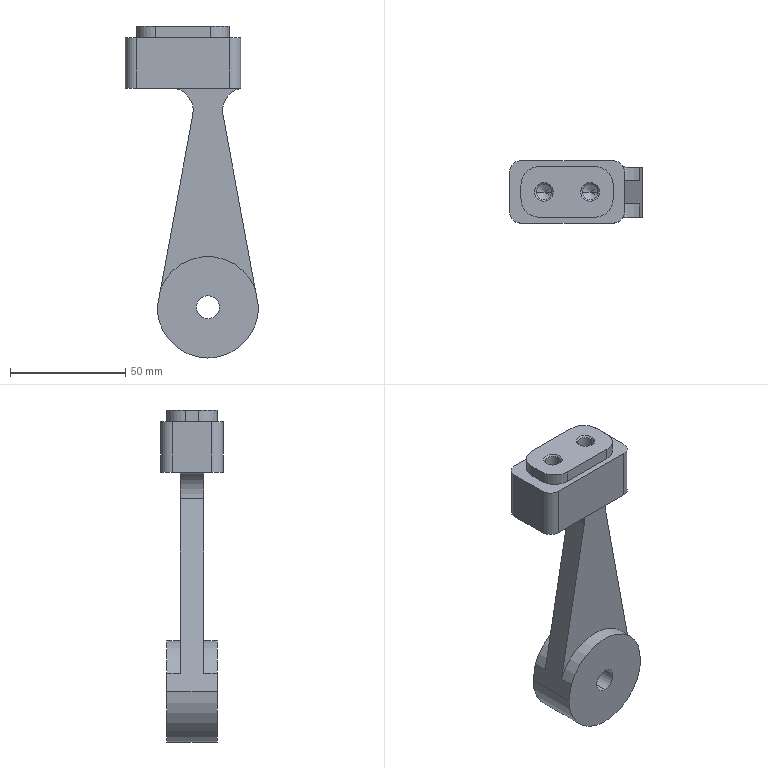Part | SolidWorks | features ICE 3, 3DProfileFeature 1, Extrusion 1, HoleWzd 1 | 1 solid | 45 faces | box 57.8 x 27 x 144 mm | volume 81593 mm3 | cylinder 20 | plane 17 | cone 8 | commonest cylinder face diameters 10 x6 6.8 x4 16 x4 44 x4 20 x2
STEP:
#1=CARTESIAN_POINT('',(-13.4,0.,26.375));
#2=VERTEX_POINT('',#1);
#3=CARTESIAN_POINT('',(-6.6,0.,26.375));
#4=VERTEX_POINT('',#3);
#5=CARTESIAN_POINT('',(-10.,0.,26.375));
#6=DIRECTION('',(0.,0.,1.));
#7=DIRECTION('',(1.,0.,0.));
#8=AXIS2_PLACEMENT_3D('',#5,#6,#7);
#9=CIRCLE('',#8,3.4);
#10=EDGE_CURVE('',#2,#4,#9,.T.);
#11=ORIENTED_EDGE('',*,*,#10,.F.);
#12=CARTESIAN_POINT('',(-14.025,0.,27.));
#13=VERTEX_POINT('',#12);
#14=CARTESIAN_POINT('',(-14.025,0.,27.));
#15=DIRECTION('',(-0.7071,0.,0.7071));
#16=VECTOR('',#15,1000.);
#17=LINE('',#14,#16);
#18=EDGE_CURVE('',#2,#13,#17,.T.);
#19=ORIENTED_EDGE('',*,*,#18,.T.);
#20=CARTESIAN_POINT('',(-5.975,0.,27.));
#21=VERTEX_POINT('',#20);
#22=CARTESIAN_POINT('',(-10.,0.,27.));
#23=DIRECTION('',(0.,0.,1.));
#24=DIRECTION('',(1.,0.,0.));
#25=AXIS2_PLACEMENT_3D('',#22,#23,#24);
#26=CIRCLE('',#25,4.025);
#27=EDGE_CURVE('',#13,#21,#26,.T.);
#28=ORIENTED_EDGE('',*,*,#27,.T.);
#29=CARTESIAN_POINT('',(-5.975,0.,27.));
#30=DIRECTION('',(0.7071,0.,0.7071));
#31=VECTOR('',#30,1000.);
#32=LINE('',#29,#31);
#33=EDGE_CURVE('',#4,#21,#32,.T.);
#34=ORIENTED_EDGE('',*,*,#33,.F.);
#35=EDGE_LOOP('',(#11,#19,#28,#34));
#36=FACE_OUTER_BOUND('',#35,.T.);
#37=CARTESIAN_POINT('',(-10.,0.,27.));
#38=DIRECTION('',(0.,0.,1.));
#39=DIRECTION('',(1.,0.,0.));
#40=AXIS2_PLACEMENT_3D('',#37,#38,#39);
#41=CONICAL_SURFACE('',#40,4.025,0.7854);
#42=ADVANCED_FACE('',(#36),#41,.F.);
#43=CARTESIAN_POINT('',(-13.4,0.,7.043));
#44=VERTEX_POINT('',#43);
#45=CARTESIAN_POINT('',(-6.6,0.,7.043));
#46=VERTEX_POINT('',#45);
#47=CARTESIAN_POINT('',(-10.,0.,7.043));
#48=DIRECTION('',(0.,0.,1.));
#49=DIRECTION('',(1.,0.,0.));
#50=AXIS2_PLACEMENT_3D('',#47,#48,#49);
#51=CIRCLE('',#50,3.4);
#52=EDGE_CURVE('',#44,#46,#51,.T.);
#53=ORIENTED_EDGE('',*,*,#52,.F.);
#54=CARTESIAN_POINT('',(-13.4,0.,27.));
#55=DIRECTION('',(0.,0.,1.));
#56=VECTOR('',#55,1000.);
#57=LINE('',#54,#56);
#58=EDGE_CURVE('',#44,#2,#57,.T.);
#59=ORIENTED_EDGE('',*,*,#58,.T.);
#60=ORIENTED_EDGE('',*,*,#10,.T.);
#61=CARTESIAN_POINT('',(-6.6,0.,27.));
#62=DIRECTION('',(0.,0.,1.));
#63=VECTOR('',#62,1000.);
#64=LINE('',#61,#63);
#65=EDGE_CURVE('',#46,#4,#64,.T.);
#66=ORIENTED_EDGE('',*,*,#65,.F.);
#67=EDGE_LOOP('',(#53,#59,#60,#66));
#68=FACE_OUTER_BOUND('',#67,.T.);
#69=CARTESIAN_POINT('',(-10.,0.,27.));
#70=DIRECTION('',(0.,0.,1.));
#71=DIRECTION('',(1.,0.,0.));
#72=AXIS2_PLACEMENT_3D('',#69,#70,#71);
#73=CYLINDRICAL_SURFACE('',#72,3.4);
#74=ADVANCED_FACE('',(#68),#73,.F.);
#75=CARTESIAN_POINT('',(-10.,0.,5.));
#76=VERTEX_POINT('',#75);
#77=CARTESIAN_POINT('',(-6.6,0.,7.043));
#78=DIRECTION('',(0.8572,0.,0.515));
#79=VECTOR('',#78,1000.);
#80=LINE('',#77,#79);
#81=EDGE_CURVE('',#76,#46,#80,.T.);
#82=ORIENTED_EDGE('',*,*,#81,.F.);
#83=CARTESIAN_POINT('',(-13.4,0.,7.043));
#84=DIRECTION('',(-0.8572,0.,0.515));
#85=VECTOR('',#84,1000.);
#86=LINE('',#83,#85);
#87=EDGE_CURVE('',#76,#44,#86,.T.);
#88=ORIENTED_EDGE('',*,*,#87,.T.);
#89=ORIENTED_EDGE('',*,*,#52,.T.);
#90=EDGE_LOOP('',(#82,#88,#89));
#91=FACE_OUTER_BOUND('',#90,.T.);
#92=CARTESIAN_POINT('',(-10.,0.,7.043));
#93=DIRECTION('',(0.,0.,1.));
#94=DIRECTION('',(1.,0.,0.));
#95=AXIS2_PLACEMENT_3D('',#92,#93,#94);
#96=CONICAL_SURFACE('',#95,3.4,1.03);
#97=ADVANCED_FACE('',(#91),#96,.F.);
#98=CARTESIAN_POINT('',(6.6,0.,26.375));
#99=VERTEX_POINT('',#98);
#100=CARTESIAN_POINT('',(13.4,0.,26.375));
#101=VERTEX_POINT('',#100);
#102=CARTESIAN_POINT('',(10.,0.,26.375));
#103=DIRECTION('',(0.,0.,1.));
#104=DIRECTION('',(1.,0.,0.));
#105=AXIS2_PLACEMENT_3D('',#102,#103,#104);
#106=CIRCLE('',#105,3.4);
#107=EDGE_CURVE('',#99,#101,#106,.T.);
#108=ORIENTED_EDGE('',*,*,#107,.F.);
#109=CARTESIAN_POINT('',(5.975,0.,27.));
#110=VERTEX_POINT('',#109);
#111=CARTESIAN_POINT('',(5.975,0.,27.));
#112=DIRECTION('',(-0.7071,0.,0.7071));
#113=VECTOR('',#112,1000.);
#114=LINE('',#111,#113);
#115=EDGE_CURVE('',#99,#110,#114,.T.);
#116=ORIENTED_EDGE('',*,*,#115,.T.);
#117=CARTESIAN_POINT('',(14.025,0.,27.));
#118=VERTEX_POINT('',#117);
#119=CARTESIAN_POINT('',(10.,0.,27.));
#120=DIRECTION('',(0.,0.,1.));
#121=DIRECTION('',(1.,0.,0.));
#122=AXIS2_PLACEMENT_3D('',#119,#120,#121);
#123=CIRCLE('',#122,4.025);
#124=EDGE_CURVE('',#110,#118,#123,.T.);
#125=ORIENTED_EDGE('',*,*,#124,.T.);
#126=CARTESIAN_POINT('',(14.025,0.,27.));
#127=DIRECTION('',(0.7071,0.,0.7071));
#128=VECTOR('',#127,1000.);
#129=LINE('',#126,#128);
#130=EDGE_CURVE('',#101,#118,#129,.T.);
#131=ORIENTED_EDGE('',*,*,#130,.F.);
#132=EDGE_LOOP('',(#108,#116,#125,#131));
#133=FACE_OUTER_BOUND('',#132,.T.);
#134=CARTESIAN_POINT('',(10.,0.,27.));
#135=DIRECTION('',(0.,0.,1.));
#136=DIRECTION('',(1.,0.,0.));
#137=AXIS2_PLACEMENT_3D('',#134,#135,#136);
#138=CONICAL_SURFACE('',#137,4.025,0.7854);
#139=ADVANCED_FACE('',(#133),#138,.F.);
#140=CARTESIAN_POINT('',(6.6,0.,7.043));
#141=VERTEX_POINT('',#140);
#142=CARTESIAN_POINT('',(13.4,0.,7.043));
#143=VERTEX_POINT('',#142);
#144=CARTESIAN_POINT('',(10.,0.,7.043));
#145=DIRECTION('',(0.,0.,1.));
#146=DIRECTION('',(1.,0.,0.));
#147=AXIS2_PLACEMENT_3D('',#144,#145,#146);
#148=CIRCLE('',#147,3.4);
#149=EDGE_CURVE('',#141,#143,#148,.T.);
#150=ORIENTED_EDGE('',*,*,#149,.F.);
#151=CARTESIAN_POINT('',(6.6,0.,27.));
#152=DIRECTION('',(0.,0.,1.));
#153=VECTOR('',#152,1000.);
#154=LINE('',#151,#153);
#155=EDGE_CURVE('',#141,#99,#154,.T.);
#156=ORIENTED_EDGE('',*,*,#155,.T.);
#157=ORIENTED_EDGE('',*,*,#107,.T.);
#158=CARTESIAN_POINT('',(13.4,0.,27.));
#159=DIRECTION('',(0.,0.,1.));
#160=VECTOR('',#159,1000.);
#161=LINE('',#158,#160);
#162=EDGE_CURVE('',#143,#101,#161,.T.);
#163=ORIENTED_EDGE('',*,*,#162,.F.);
#164=EDGE_LOOP('',(#150,#156,#157,#163));
#165=FACE_OUTER_BOUND('',#164,.T.);
#166=CARTESIAN_POINT('',(10.,0.,27.));
#167=DIRECTION('',(0.,0.,1.));
#168=DIRECTION('',(1.,0.,0.));
#169=AXIS2_PLACEMENT_3D('',#166,#167,#168);
#170=CYLINDRICAL_SURFACE('',#169,3.4);
#171=ADVANCED_FACE('',(#165),#170,.F.);
#172=CARTESIAN_POINT('',(10.,0.,5.));
#173=VERTEX_POINT('',#172);
#174=CARTESIAN_POINT('',(13.4,0.,7.043));
#175=DIRECTION('',(0.8572,0.,0.515));
#176=VECTOR('',#175,1000.);
#177=LINE('',#174,#176);
#178=EDGE_CURVE('',#173,#143,#177,.T.);
#179=ORIENTED_EDGE('',*,*,#178,.F.);
#180=CARTESIAN_POINT('',(6.6,0.,7.043));
#181=DIRECTION('',(-0.8572,0.,0.515));
#182=VECTOR('',#181,1000.);
#183=LINE('',#180,#182);
#184=EDGE_CURVE('',#173,#141,#183,.T.);
#185=ORIENTED_EDGE('',*,*,#184,.T.);
#186=ORIENTED_EDGE('',*,*,#149,.T.);
#187=EDGE_LOOP('',(#179,#185,#186));
#188=FACE_OUTER_BOUND('',#187,.T.);
#189=CARTESIAN_POINT('',(10.,0.,7.043));
#190=DIRECTION('',(0.,0.,1.));
#191=DIRECTION('',(1.,0.,0.));
#192=AXIS2_PLACEMENT_3D('',#189,#190,#191);
#193=CONICAL_SURFACE('',#192,3.4,1.03);
#194=ADVANCED_FACE('',(#188),#193,.F.);
#195=CARTESIAN_POINT('',(10.8,11.,-100.));
#196=VERTEX_POINT('',#195);
#197=CARTESIAN_POINT('',(10.8,11.,-90.));
#198=VERTEX_POINT('',#197);
#199=CARTESIAN_POINT('',(10.8,11.,-95.));
#200=DIRECTION('',(0.,1.,0.));
#201=DIRECTION('',(0.,0.,1.));
#202=AXIS2_PLACEMENT_3D('',#199,#200,#201);
#203=CIRCLE('',#202,5.);
#204=EDGE_CURVE('',#196,#198,#203,.T.);
#205=ORIENTED_EDGE('',*,*,#204,.T.);
#206=CARTESIAN_POINT('',(10.8,-11.,-90.));
#207=VERTEX_POINT('',#206);
#208=CARTESIAN_POINT('',(10.8,11.,-90.));
#209=DIRECTION('',(0.,-1.,0.));
#210=VECTOR('',#209,1000.);
#211=LINE('',#208,#210);
#212=EDGE_CURVE('',#198,#207,#211,.T.);
#213=ORIENTED_EDGE('',*,*,#212,.T.);
#214=CARTESIAN_POINT('',(10.8,-11.,-100.));
#215=VERTEX_POINT('',#214);
#216=CARTESIAN_POINT('',(10.8,-11.,-95.));
#217=DIRECTION('',(0.,1.,0.));
#218=DIRECTION('',(0.,0.,1.));
#219=AXIS2_PLACEMENT_3D('',#216,#217,#218);
#220=CIRCLE('',#219,5.);
#221=EDGE_CURVE('',#215,#207,#220,.T.);
#222=ORIENTED_EDGE('',*,*,#221,.F.);
#223=CARTESIAN_POINT('',(10.8,11.,-100.));
#224=DIRECTION('',(0.,-1.,0.));
#225=VECTOR('',#224,1000.);
#226=LINE('',#223,#225);
#227=EDGE_CURVE('',#196,#215,#226,.T.);
#228=ORIENTED_EDGE('',*,*,#227,.F.);
#229=EDGE_LOOP('',(#205,#213,#222,#228));
#230=FACE_OUTER_BOUND('',#229,.T.);
#231=CARTESIAN_POINT('',(10.8,11.,-95.));
#232=DIRECTION('',(0.,-1.,0.));
#233=DIRECTION('',(0.,0.,-1.));
#234=AXIS2_PLACEMENT_3D('',#231,#232,#233);
#235=CYLINDRICAL_SURFACE('',#234,5.);
#236=ADVANCED_FACE('',(#230),#235,.F.);
#237=CARTESIAN_POINT('',(10.8,11.,-117.));
#238=VERTEX_POINT('',#237);
#239=CARTESIAN_POINT('',(-11.2,11.,-95.));
#240=VERTEX_POINT('',#239);
#241=CARTESIAN_POINT('',(10.8,11.,-95.));
#242=DIRECTION('',(0.,1.,0.));
#243=DIRECTION('',(0.,0.,1.));
#244=AXIS2_PLACEMENT_3D('',#241,#242,#243);
#245=CIRCLE('',#244,22.);
#246=EDGE_CURVE('',#238,#240,#245,.T.);
#247=ORIENTED_EDGE('',*,*,#246,.F.);
#248=CARTESIAN_POINT('',(10.8,-11.,-117.));
#249=VERTEX_POINT('',#248);
#250=CARTESIAN_POINT('',(10.8,11.,-117.));
#251=DIRECTION('',(0.,-1.,0.));
#252=VECTOR('',#251,1000.);
#253=LINE('',#250,#252);
#254=EDGE_CURVE('',#238,#249,#253,.T.);
#255=ORIENTED_EDGE('',*,*,#254,.T.);
#256=CARTESIAN_POINT('',(-11.2,-11.,-95.));
#257=VERTEX_POINT('',#256);
#258=CARTESIAN_POINT('',(10.8,-11.,-95.));
#259=DIRECTION('',(0.,1.,0.));
#260=DIRECTION('',(0.,0.,1.));
#261=AXIS2_PLACEMENT_3D('',#258,#259,#260);
#262=CIRCLE('',#261,22.);
#263=EDGE_CURVE('',#249,#257,#262,.T.);
#264=ORIENTED_EDGE('',*,*,#263,.T.);
#265=CARTESIAN_POINT('',(-11.2,11.,-95.));
#266=DIRECTION('',(0.,-1.,0.));
#267=VECTOR('',#266,1000.);
#268=LINE('',#265,#267);
#269=EDGE_CURVE('',#240,#257,#268,.T.);
#270=ORIENTED_EDGE('',*,*,#269,.F.);
#271=EDGE_LOOP('',(#247,#255,#264,#270));
#272=FACE_OUTER_BOUND('',#271,.T.);
#273=CARTESIAN_POINT('',(10.8,11.,-95.));
#274=DIRECTION('',(0.,-1.,0.));
#275=DIRECTION('',(0.,0.,-1.));
#276=AXIS2_PLACEMENT_3D('',#273,#274,#275);
#277=CYLINDRICAL_SURFACE('',#276,22.);
#278=ADVANCED_FACE('',(#272),#277,.T.);
#279=CARTESIAN_POINT('',(-3.4,5.,0.));
#280=VERTEX_POINT('',#279);
#281=CARTESIAN_POINT('',(-3.4,-5.,0.));
#282=VERTEX_POINT('',#281);
#283=CARTESIAN_POINT('',(-3.4,5.,0.));
#284=DIRECTION('',(0.,-1.,0.));
#285=VECTOR('',#284,1000.);
#286=LINE('',#283,#285);
#287=EDGE_CURVE('',#280,#282,#286,.T.);
#288=ORIENTED_EDGE('',*,*,#287,.T.);
#289=CARTESIAN_POINT('',(25.,-5.,0.));
#290=VERTEX_POINT('',#289);
#291=CARTESIAN_POINT('',(0.,-5.,0.));
#292=DIRECTION('',(1.,0.,0.));
#293=VECTOR('',#292,1000.);
#294=LINE('',#291,#293);
#295=EDGE_CURVE('',#282,#290,#294,.T.);
#296=ORIENTED_EDGE('',*,*,#295,.T.);
#297=CARTESIAN_POINT('',(25.,-8.5,0.));
#298=VERTEX_POINT('',#297);
#299=CARTESIAN_POINT('',(25.,-8.5,0.));
#300=DIRECTION('',(0.,1.,0.));
#301=VECTOR('',#300,1000.);
#302=LINE('',#299,#301);
#303=EDGE_CURVE('',#298,#290,#302,.T.);
#304=ORIENTED_EDGE('',*,*,#303,.F.);
#305=CARTESIAN_POINT('',(20.,-13.5,0.));
#306=VERTEX_POINT('',#305);
#307=CARTESIAN_POINT('',(20.,-8.5,0.));
#308=DIRECTION('',(0.,0.,1.));
#309=DIRECTION('',(1.,0.,0.));
#310=AXIS2_PLACEMENT_3D('',#307,#308,#309);
#311=CIRCLE('',#310,5.);
#312=EDGE_CURVE('',#306,#298,#311,.T.);
#313=ORIENTED_EDGE('',*,*,#312,.F.);
#314=CARTESIAN_POINT('',(-20.,-13.5,0.));
#315=VERTEX_POINT('',#314);
#316=CARTESIAN_POINT('',(-20.,-13.5,0.));
#317=DIRECTION('',(1.,0.,0.));
#318=VECTOR('',#317,1000.);
#319=LINE('',#316,#318);
#320=EDGE_CURVE('',#315,#306,#319,.T.);
#321=ORIENTED_EDGE('',*,*,#320,.F.);
#322=CARTESIAN_POINT('',(-25.,-8.5,0.));
#323=VERTEX_POINT('',#322);
#324=CARTESIAN_POINT('',(-20.,-8.5,0.));
#325=DIRECTION('',(0.,0.,1.));
#326=DIRECTION('',(-1.,0.,0.));
#327=AXIS2_PLACEMENT_3D('',#324,#325,#326);
#328=CIRCLE('',#327,5.);
#329=EDGE_CURVE('',#323,#315,#328,.T.);
#330=ORIENTED_EDGE('',*,*,#329,.F.);
#331=CARTESIAN_POINT('',(-25.,8.5,0.));
#332=VERTEX_POINT('',#331);
#333=CARTESIAN_POINT('',(-25.,-8.5,0.));
#334=DIRECTION('',(0.,-1.,0.));
#335=VECTOR('',#334,1000.);
#336=LINE('',#333,#335);
#337=EDGE_CURVE('',#332,#323,#336,.T.);
#338=ORIENTED_EDGE('',*,*,#337,.F.);
#339=CARTESIAN_POINT('',(-20.,13.5,0.));
#340=VERTEX_POINT('',#339);
#341=CARTESIAN_POINT('',(-20.,8.5,0.));
#342=DIRECTION('',(0.,0.,1.));
#343=DIRECTION('',(-1.,0.,0.));
#344=AXIS2_PLACEMENT_3D('',#341,#342,#343);
#345=CIRCLE('',#344,5.);
#346=EDGE_CURVE('',#340,#332,#345,.T.);
#347=ORIENTED_EDGE('',*,*,#346,.F.);
#348=CARTESIAN_POINT('',(20.,13.5,0.));
#349=VERTEX_POINT('',#348);
#350=CARTESIAN_POINT('',(-20.,13.5,0.));
#351=DIRECTION('',(-1.,0.,0.));
#352=VECTOR('',#351,1000.);
#353=LINE('',#350,#352);
#354=EDGE_CURVE('',#349,#340,#353,.T.);
#355=ORIENTED_EDGE('',*,*,#354,.F.);
#356=CARTESIAN_POINT('',(25.,8.5,0.));
#357=VERTEX_POINT('',#356);
#358=CARTESIAN_POINT('',(20.,8.5,0.));
#359=DIRECTION('',(0.,0.,1.));
#360=DIRECTION('',(-1.,0.,0.));
#361=AXIS2_PLACEMENT_3D('',#358,#359,#360);
#362=CIRCLE('',#361,5.);
#363=EDGE_CURVE('',#357,#349,#362,.T.);
#364=ORIENTED_EDGE('',*,*,#363,.F.);
#365=CARTESIAN_POINT('',(25.,5.,0.));
#366=VERTEX_POINT('',#365);
#367=CARTESIAN_POINT('',(25.,-8.5,0.));
#368=DIRECTION('',(0.,1.,0.));
#369=VECTOR('',#368,1000.);
#370=LINE('',#367,#369);
#371=EDGE_CURVE('',#366,#357,#370,.T.);
#372=ORIENTED_EDGE('',*,*,#371,.F.);
#373=CARTESIAN_POINT('',(0.,5.,0.));
#374=DIRECTION('',(1.,0.,0.));
#375=VECTOR('',#374,1000.);
#376=LINE('',#373,#375);
#377=EDGE_CURVE('',#280,#366,#376,.T.);
#378=ORIENTED_EDGE('',*,*,#377,.F.);
#379=EDGE_LOOP('',(#288,#296,#304,#313,#321,#330,#338,#347,#355,#364,#372,#378));
#380=FACE_OUTER_BOUND('',#379,.T.);
#381=CARTESIAN_POINT('',(-20.,8.5,0.));
#382=DIRECTION('',(0.,0.,-1.));
#383=DIRECTION('',(-1.,0.,0.));
#384=AXIS2_PLACEMENT_3D('',#381,#382,#383);
#385=PLANE('',#384);
#386=ADVANCED_FACE('',(#380),#385,.T.);
#387=CARTESIAN_POINT('',(-20.,13.5,22.));
#388=VERTEX_POINT('',#387);
#389=CARTESIAN_POINT('',(-25.,8.5,22.));
#390=VERTEX_POINT('',#389);
#391=CARTESIAN_POINT('',(-20.,8.5,22.));
#392=DIRECTION('',(0.,0.,1.));
#393=DIRECTION('',(-1.,0.,0.));
#394=AXIS2_PLACEMENT_3D('',#391,#392,#393);
#395=CIRCLE('',#394,5.);
#396=EDGE_CURVE('',#388,#390,#395,.T.);
#397=ORIENTED_EDGE('',*,*,#396,.T.);
#398=CARTESIAN_POINT('',(-25.,-8.5,22.));
#399=VERTEX_POINT('',#398);
#400=CARTESIAN_POINT('',(-25.,-8.5,22.));
#401=DIRECTION('',(0.,-1.,0.));
#402=VECTOR('',#401,1000.);
#403=LINE('',#400,#402);
#404=EDGE_CURVE('',#390,#399,#403,.T.);
#405=ORIENTED_EDGE('',*,*,#404,.T.);
#406=CARTESIAN_POINT('',(-20.,-13.5,22.));
#407=VERTEX_POINT('',#406);
#408=CARTESIAN_POINT('',(-20.,-8.5,22.));
#409=DIRECTION('',(0.,0.,1.));
#410=DIRECTION('',(-1.,0.,0.));
#411=AXIS2_PLACEMENT_3D('',#408,#409,#410);
#412=CIRCLE('',#411,5.);
#413=EDGE_CURVE('',#399,#407,#412,.T.);
#414=ORIENTED_EDGE('',*,*,#413,.T.);
#415=CARTESIAN_POINT('',(20.,-13.5,22.));
#416=VERTEX_POINT('',#415);
#417=CARTESIAN_POINT('',(-20.,-13.5,22.));
#418=DIRECTION('',(1.,0.,0.));
#419=VECTOR('',#418,1000.);
#420=LINE('',#417,#419);
#421=EDGE_CURVE('',#407,#416,#420,.T.);
#422=ORIENTED_EDGE('',*,*,#421,.T.);
#423=CARTESIAN_POINT('',(25.,-8.5,22.));
#424=VERTEX_POINT('',#423);
#425=CARTESIAN_POINT('',(20.,-8.5,22.));
#426=DIRECTION('',(0.,0.,1.));
#427=DIRECTION('',(1.,0.,0.));
#428=AXIS2_PLACEMENT_3D('',#425,#426,#427);
#429=CIRCLE('',#428,5.);
#430=EDGE_CURVE('',#416,#424,#429,.T.);
#431=ORIENTED_EDGE('',*,*,#430,.T.);
#432=CARTESIAN_POINT('',(25.,8.5,22.));
#433=VERTEX_POINT('',#432);
#434=CARTESIAN_POINT('',(25.,-8.5,22.));
#435=DIRECTION('',(0.,1.,0.));
#436=VECTOR('',#435,1000.);
#437=LINE('',#434,#436);
#438=EDGE_CURVE('',#424,#433,#437,.T.);
#439=ORIENTED_EDGE('',*,*,#438,.T.);
#440=CARTESIAN_POINT('',(20.,13.5,22.));
#441=VERTEX_POINT('',#440);
#442=CARTESIAN_POINT('',(20.,8.5,22.));
#443=DIRECTION('',(0.,0.,1.));
#444=DIRECTION('',(-1.,0.,0.));
#445=AXIS2_PLACEMENT_3D('',#442,#443,#444);
#446=CIRCLE('',#445,5.);
#447=EDGE_CURVE('',#433,#441,#446,.T.);
#448=ORIENTED_EDGE('',*,*,#447,.T.);
#449=CARTESIAN_POINT('',(-20.,13.5,22.));
#450=DIRECTION('',(-1.,0.,0.));
#451=VECTOR('',#450,1000.);
#452=LINE('',#449,#451);
#453=EDGE_CURVE('',#441,#388,#452,.T.);
#454=ORIENTED_EDGE('',*,*,#453,.T.);
#455=EDGE_LOOP('',(#397,#405,#414,#422,#431,#439,#448,#454));
#456=FACE_OUTER_BOUND('',#455,.T.);
#457=CARTESIAN_POINT('',(12.,-11.,22.));
#458=VERTEX_POINT('',#457);
#459=CARTESIAN_POINT('',(20.,-3.,22.));
#460=VERTEX_POINT('',#459);
#461=CARTESIAN_POINT('',(12.,-3.,22.));
#462=DIRECTION('',(0.,0.,1.));
#463=DIRECTION('',(1.,0.,0.));
#464=AXIS2_PLACEMENT_3D('',#461,#462,#463);
#465=CIRCLE('',#464,8.);
#466=EDGE_CURVE('',#458,#460,#465,.T.);
#467=ORIENTED_EDGE('',*,*,#466,.F.);
#468=CARTESIAN_POINT('',(-12.,-11.,22.));
#469=VERTEX_POINT('',#468);
#470=CARTESIAN_POINT('',(-12.,-11.,22.));
#471=DIRECTION('',(1.,0.,0.));
#472=VECTOR('',#471,1000.);
#473=LINE('',#470,#472);
#474=EDGE_CURVE('',#469,#458,#473,.T.);
#475=ORIENTED_EDGE('',*,*,#474,.F.);
#476=CARTESIAN_POINT('',(-20.,-3.,22.));
#477=VERTEX_POINT('',#476);
#478=CARTESIAN_POINT('',(-12.,-3.,22.));
#479=DIRECTION('',(0.,0.,1.));
#480=DIRECTION('',(-1.,0.,0.));
#481=AXIS2_PLACEMENT_3D('',#478,#479,#480);
#482=CIRCLE('',#481,8.);
#483=EDGE_CURVE('',#477,#469,#482,.T.);
#484=ORIENTED_EDGE('',*,*,#483,.F.);
#485=CARTESIAN_POINT('',(-20.,3.,22.));
#486=VERTEX_POINT('',#485);
#487=CARTESIAN_POINT('',(-20.,-3.,22.));
#488=DIRECTION('',(0.,-1.,0.));
#489=VECTOR('',#488,1000.);
#490=LINE('',#487,#489);
#491=EDGE_CURVE('',#486,#477,#490,.T.);
#492=ORIENTED_EDGE('',*,*,#491,.F.);
#493=CARTESIAN_POINT('',(-12.,11.,22.));
#494=VERTEX_POINT('',#493);
#495=CARTESIAN_POINT('',(-12.,3.,22.));
#496=DIRECTION('',(0.,0.,1.));
#497=DIRECTION('',(-1.,0.,0.));
#498=AXIS2_PLACEMENT_3D('',#495,#496,#497);
#499=CIRCLE('',#498,8.);
#500=EDGE_CURVE('',#494,#486,#499,.T.);
#501=ORIENTED_EDGE('',*,*,#500,.F.);
#502=CARTESIAN_POINT('',(12.,11.,22.));
#503=VERTEX_POINT('',#502);
#504=CARTESIAN_POINT('',(-12.,11.,22.));
#505=DIRECTION('',(-1.,0.,0.));
#506=VECTOR('',#505,1000.);
#507=LINE('',#504,#506);
#508=EDGE_CURVE('',#503,#494,#507,.T.);
#509=ORIENTED_EDGE('',*,*,#508,.F.);
#510=CARTESIAN_POINT('',(20.,3.,22.));
#511=VERTEX_POINT('',#510);
#512=CARTESIAN_POINT('',(12.,3.,22.));
#513=DIRECTION('',(0.,0.,1.));
#514=DIRECTION('',(-1.,0.,0.));
#515=AXIS2_PLACEMENT_3D('',#512,#513,#514);
#516=CIRCLE('',#515,8.);
#517=EDGE_CURVE('',#511,#503,#516,.T.);
#518=ORIENTED_EDGE('',*,*,#517,.F.);
#519=CARTESIAN_POINT('',(20.,-3.,22.));
#520=DIRECTION('',(0.,1.,0.));
#521=VECTOR('',#520,1000.);
#522=LINE('',#519,#521);
#523=EDGE_CURVE('',#460,#511,#522,.T.);
#524=ORIENTED_EDGE('',*,*,#523,.F.);
#525=EDGE_LOOP('',(#467,#475,#484,#492,#501,#509,#518,#524));
#526=FACE_BOUND('',#525,.T.);
#527=CARTESIAN_POINT('',(-20.,8.5,22.));
#528=DIRECTION('',(0.,0.,-1.));
#529=DIRECTION('',(-1.,0.,0.));
#530=AXIS2_PLACEMENT_3D('',#527,#528,#529);
#531=PLANE('',#530);
#532=ADVANCED_FACE('',(#456,#526),#531,.F.);
#533=ORIENTED_EDGE('',*,*,#346,.T.);
#534=CARTESIAN_POINT('',(-25.,8.5,22.));
#535=DIRECTION('',(0.,0.,-1.));
#536=VECTOR('',#535,1000.);
#537=LINE('',#534,#536);
#538=EDGE_CURVE('',#390,#332,#537,.T.);
#539=ORIENTED_EDGE('',*,*,#538,.F.);
#540=ORIENTED_EDGE('',*,*,#396,.F.);
#541=CARTESIAN_POINT('',(-20.,13.5,22.));
#542=DIRECTION('',(0.,0.,-1.));
#543=VECTOR('',#542,1000.);
#544=LINE('',#541,#543);
#545=EDGE_CURVE('',#388,#340,#544,.T.);
#546=ORIENTED_EDGE('',*,*,#545,.T.);
#547=EDGE_LOOP('',(#533,#539,#540,#546));
#548=FACE_OUTER_BOUND('',#547,.T.);
#549=CARTESIAN_POINT('',(-20.,8.5,22.));
#550=DIRECTION('',(0.,0.,-1.));
#551=DIRECTION('',(-1.,0.,0.));
#552=AXIS2_PLACEMENT_3D('',#549,#550,#551);
#553=CYLINDRICAL_SURFACE('',#552,5.);
#554=ADVANCED_FACE('',(#548),#553,.T.);
#555=ORIENTED_EDGE('',*,*,#337,.T.);
#556=CARTESIAN_POINT('',(-25.,-8.5,22.));
#557=DIRECTION('',(0.,0.,-1.));
#558=VECTOR('',#557,1000.);
#559=LINE('',#556,#558);
#560=EDGE_CURVE('',#399,#323,#559,.T.);
#561=ORIENTED_EDGE('',*,*,#560,.F.);
#562=ORIENTED_EDGE('',*,*,#404,.F.);
#563=ORIENTED_EDGE('',*,*,#538,.T.);
#564=EDGE_LOOP('',(#555,#561,#562,#563));
#565=FACE_OUTER_BOUND('',#564,.T.);
#566=CARTESIAN_POINT('',(-25.,-8.5,22.));
#567=DIRECTION('',(1.,0.,0.));
#568=DIRECTION('',(0.,0.,-1.));
#569=AXIS2_PLACEMENT_3D('',#566,#567,#568);
#570=PLANE('',#569);
#571=ADVANCED_FACE('',(#565),#570,.F.);
#572=ORIENTED_EDGE('',*,*,#329,.T.);
#573=CARTESIAN_POINT('',(-20.,-13.5,22.));
#574=DIRECTION('',(0.,0.,-1.));
#575=VECTOR('',#574,1000.);
#576=LINE('',#573,#575);
#577=EDGE_CURVE('',#407,#315,#576,.T.);
#578=ORIENTED_EDGE('',*,*,#577,.F.);
#579=ORIENTED_EDGE('',*,*,#413,.F.);
#580=ORIENTED_EDGE('',*,*,#560,.T.);
#581=EDGE_LOOP('',(#572,#578,#579,#580));
#582=FACE_OUTER_BOUND('',#581,.T.);
#583=CARTESIAN_POINT('',(-20.,-8.5,22.));
#584=DIRECTION('',(0.,0.,-1.));
#585=DIRECTION('',(-1.,0.,0.));
#586=AXIS2_PLACEMENT_3D('',#583,#584,#585);
#587=CYLINDRICAL_SURFACE('',#586,5.);
#588=ADVANCED_FACE('',(#582),#587,.T.);
#589=ORIENTED_EDGE('',*,*,#320,.T.);
#590=CARTESIAN_POINT('',(20.,-13.5,22.));
#591=DIRECTION('',(0.,0.,-1.));
#592=VECTOR('',#591,1000.);
#593=LINE('',#590,#592);
#594=EDGE_CURVE('',#416,#306,#593,.T.);
#595=ORIENTED_EDGE('',*,*,#594,.F.);
#596=ORIENTED_EDGE('',*,*,#421,.F.);
#597=ORIENTED_EDGE('',*,*,#577,.T.);
#598=EDGE_LOOP('',(#589,#595,#596,#597));
#599=FACE_OUTER_BOUND('',#598,.T.);
#600=CARTESIAN_POINT('',(-20.,-13.5,22.));
#601=DIRECTION('',(0.,1.,0.));
#602=DIRECTION('',(0.,0.,1.));
#603=AXIS2_PLACEMENT_3D('',#600,#601,#602);
#604=PLANE('',#603);
#605=ADVANCED_FACE('',(#599),#604,.F.);
#606=ORIENTED_EDGE('',*,*,#312,.T.);
#607=CARTESIAN_POINT('',(25.,-8.5,22.));
#608=DIRECTION('',(0.,0.,-1.));
#609=VECTOR('',#608,1000.);
#610=LINE('',#607,#609);
#611=EDGE_CURVE('',#424,#298,#610,.T.);
#612=ORIENTED_EDGE('',*,*,#611,.F.);
#613=ORIENTED_EDGE('',*,*,#430,.F.);
#614=ORIENTED_EDGE('',*,*,#594,.T.);
#615=EDGE_LOOP('',(#606,#612,#613,#614));
#616=FACE_OUTER_BOUND('',#615,.T.);
#617=CARTESIAN_POINT('',(20.,-8.5,22.));
#618=DIRECTION('',(0.,0.,-1.));
#619=DIRECTION('',(-1.,0.,0.));
#620=AXIS2_PLACEMENT_3D('',#617,#618,#619);
#621=CYLINDRICAL_SURFACE('',#620,5.);
#622=ADVANCED_FACE('',(#616),#621,.T.);
#623=ORIENTED_EDGE('',*,*,#303,.T.);
#624=CARTESIAN_POINT('',(25.,5.,0.));
#625=DIRECTION('',(0.,-1.,0.));
#626=VECTOR('',#625,1000.);
#627=LINE('',#624,#626);
#628=EDGE_CURVE('',#366,#290,#627,.T.);
#629=ORIENTED_EDGE('',*,*,#628,.F.);
#630=ORIENTED_EDGE('',*,*,#371,.T.);
#631=CARTESIAN_POINT('',(25.,8.5,22.));
#632=DIRECTION('',(0.,0.,-1.));
#633=VECTOR('',#632,1000.);
#634=LINE('',#631,#633);
#635=EDGE_CURVE('',#433,#357,#634,.T.);
#636=ORIENTED_EDGE('',*,*,#635,.F.);
#637=ORIENTED_EDGE('',*,*,#438,.F.);
#638=ORIENTED_EDGE('',*,*,#611,.T.);
#639=EDGE_LOOP('',(#623,#629,#630,#636,#637,#638));
#640=FACE_OUTER_BOUND('',#639,.T.);
#641=CARTESIAN_POINT('',(25.,-8.5,22.));
#642=DIRECTION('',(-1.,0.,0.));
#643=DIRECTION('',(0.,0.,1.));
#644=AXIS2_PLACEMENT_3D('',#641,#642,#643);
#645=PLANE('',#644);
#646=ADVANCED_FACE('',(#640),#645,.F.);
#647=ORIENTED_EDGE('',*,*,#363,.T.);
#648=CARTESIAN_POINT('',(20.,13.5,22.));
#649=DIRECTION('',(0.,0.,-1.));
#650=VECTOR('',#649,1000.);
#651=LINE('',#648,#650);
#652=EDGE_CURVE('',#441,#349,#651,.T.);
#653=ORIENTED_EDGE('',*,*,#652,.F.);
#654=ORIENTED_EDGE('',*,*,#447,.F.);
#655=ORIENTED_EDGE('',*,*,#635,.T.);
#656=EDGE_LOOP('',(#647,#653,#654,#655));
#657=FACE_OUTER_BOUND('',#656,.T.);
#658=CARTESIAN_POINT('',(20.,8.5,22.));
#659=DIRECTION('',(0.,0.,-1.));
#660=DIRECTION('',(-1.,0.,0.));
#661=AXIS2_PLACEMENT_3D('',#658,#659,#660);
#662=CYLINDRICAL_SURFACE('',#661,5.);
#663=ADVANCED_FACE('',(#657),#662,.T.);
#664=ORIENTED_EDGE('',*,*,#354,.T.);
#665=ORIENTED_EDGE('',*,*,#545,.F.);
#666=ORIENTED_EDGE('',*,*,#453,.F.);
#667=ORIENTED_EDGE('',*,*,#652,.T.);
#668=EDGE_LOOP('',(#664,#665,#666,#667));
#669=FACE_OUTER_BOUND('',#668,.T.);
#670=CARTESIAN_POINT('',(-20.,13.5,22.));
#671=DIRECTION('',(0.,-1.,0.));
#672=DIRECTION('',(0.,0.,-1.));
#673=AXIS2_PLACEMENT_3D('',#670,#671,#672);
#674=PLANE('',#673);
#675=ADVANCED_FACE('',(#669),#674,.F.);
#676=ORIENTED_EDGE('',*,*,#466,.T.);
#677=CARTESIAN_POINT('',(20.,-3.,27.));
#678=VERTEX_POINT('',#677);
#679=CARTESIAN_POINT('',(20.,-3.,27.));
#680=DIRECTION('',(0.,0.,-1.));
#681=VECTOR('',#680,1000.);
#682=LINE('',#679,#681);
#683=EDGE_CURVE('',#678,#460,#682,.T.);
#684=ORIENTED_EDGE('',*,*,#683,.F.);
#685=CARTESIAN_POINT('',(12.,-11.,27.));
#686=VERTEX_POINT('',#685);
#687=CARTESIAN_POINT('',(12.,-3.,27.));
#688=DIRECTION('',(0.,0.,1.));
#689=DIRECTION('',(1.,0.,0.));
#690=AXIS2_PLACEMENT_3D('',#687,#688,#689);
#691=CIRCLE('',#690,8.);
#692=EDGE_CURVE('',#686,#678,#691,.T.);
#693=ORIENTED_EDGE('',*,*,#692,.F.);
#694=CARTESIAN_POINT('',(12.,-11.,27.));
#695=DIRECTION('',(0.,0.,-1.));
#696=VECTOR('',#695,1000.);
#697=LINE('',#694,#696);
#698=EDGE_CURVE('',#686,#458,#697,.T.);
#699=ORIENTED_EDGE('',*,*,#698,.T.);
#700=EDGE_LOOP('',(#676,#684,#693,#699));
#701=FACE_OUTER_BOUND('',#700,.T.);
#702=CARTESIAN_POINT('',(12.,-3.,27.));
#703=DIRECTION('',(0.,0.,-1.));
#704=DIRECTION('',(-1.,0.,0.));
#705=AXIS2_PLACEMENT_3D('',#702,#703,#704);
#706=CYLINDRICAL_SURFACE('',#705,8.);
#707=ADVANCED_FACE('',(#701),#706,.T.);
#708=ORIENTED_EDGE('',*,*,#523,.T.);
#709=CARTESIAN_POINT('',(20.,3.,27.));
#710=VERTEX_POINT('',#709);
#711=CARTESIAN_POINT('',(20.,3.,27.));
#712=DIRECTION('',(0.,0.,-1.));
#713=VECTOR('',#712,1000.);
#714=LINE('',#711,#713);
#715=EDGE_CURVE('',#710,#511,#714,.T.);
#716=ORIENTED_EDGE('',*,*,#715,.F.);
#717=CARTESIAN_POINT('',(20.,-3.,27.));
#718=DIRECTION('',(0.,1.,0.));
#719=VECTOR('',#718,1000.);
#720=LINE('',#717,#719);
#721=EDGE_CURVE('',#678,#710,#720,.T.);
#722=ORIENTED_EDGE('',*,*,#721,.F.);
#723=ORIENTED_EDGE('',*,*,#683,.T.);
#724=EDGE_LOOP('',(#708,#716,#722,#723));
#725=FACE_OUTER_BOUND('',#724,.T.);
#726=CARTESIAN_POINT('',(20.,-3.,27.));
#727=DIRECTION('',(-1.,0.,0.));
#728=DIRECTION('',(0.,0.,1.));
#729=AXIS2_PLACEMENT_3D('',#726,#727,#728);
#730=PLANE('',#729);
#731=ADVANCED_FACE('',(#725),#730,.F.);
#732=ORIENTED_EDGE('',*,*,#517,.T.);
#733=CARTESIAN_POINT('',(12.,11.,27.));
#734=VERTEX_POINT('',#733);
#735=CARTESIAN_POINT('',(12.,11.,27.));
#736=DIRECTION('',(0.,0.,-1.));
#737=VECTOR('',#736,1000.);
#738=LINE('',#735,#737);
#739=EDGE_CURVE('',#734,#503,#738,.T.);
#740=ORIENTED_EDGE('',*,*,#739,.F.);
#741=CARTESIAN_POINT('',(12.,3.,27.));
#742=DIRECTION('',(0.,0.,1.));
#743=DIRECTION('',(-1.,0.,0.));
#744=AXIS2_PLACEMENT_3D('',#741,#742,#743);
#745=CIRCLE('',#744,8.);
#746=EDGE_CURVE('',#710,#734,#745,.T.);
#747=ORIENTED_EDGE('',*,*,#746,.F.);
#748=ORIENTED_EDGE('',*,*,#715,.T.);
#749=EDGE_LOOP('',(#732,#740,#747,#748));
#750=FACE_OUTER_BOUND('',#749,.T.);
#751=CARTESIAN_POINT('',(12.,3.,27.));
#752=DIRECTION('',(0.,0.,-1.));
#753=DIRECTION('',(-1.,0.,0.));
#754=AXIS2_PLACEMENT_3D('',#751,#752,#753);
#755=CYLINDRICAL_SURFACE('',#754,8.);
#756=ADVANCED_FACE('',(#750),#755,.T.);
#757=ORIENTED_EDGE('',*,*,#508,.T.);
#758=CARTESIAN_POINT('',(-12.,11.,27.));
#759=VERTEX_POINT('',#758);
#760=CARTESIAN_POINT('',(-12.,11.,27.));
#761=DIRECTION('',(0.,0.,-1.));
#762=VECTOR('',#761,1000.);
#763=LINE('',#760,#762);
#764=EDGE_CURVE('',#759,#494,#763,.T.);
#765=ORIENTED_EDGE('',*,*,#764,.F.);
#766=CARTESIAN_POINT('',(-12.,11.,27.));
#767=DIRECTION('',(-1.,0.,0.));
#768=VECTOR('',#767,1000.);
#769=LINE('',#766,#768);
#770=EDGE_CURVE('',#734,#759,#769,.T.);
#771=ORIENTED_EDGE('',*,*,#770,.F.);
#772=ORIENTED_EDGE('',*,*,#739,.T.);
#773=EDGE_LOOP('',(#757,#765,#771,#772));
#774=FACE_OUTER_BOUND('',#773,.T.);
#775=CARTESIAN_POINT('',(-12.,11.,27.));
#776=DIRECTION('',(0.,-1.,0.));
#777=DIRECTION('',(0.,0.,-1.));
#778=AXIS2_PLACEMENT_3D('',#775,#776,#777);
#779=PLANE('',#778);
#780=ADVANCED_FACE('',(#774),#779,.F.);
#781=ORIENTED_EDGE('',*,*,#500,.T.);
#782=CARTESIAN_POINT('',(-20.,3.,27.));
#783=VERTEX_POINT('',#782);
#784=CARTESIAN_POINT('',(-20.,3.,27.));
#785=DIRECTION('',(0.,0.,-1.));
#786=VECTOR('',#785,1000.);
#787=LINE('',#784,#786);
#788=EDGE_CURVE('',#783,#486,#787,.T.);
#789=ORIENTED_EDGE('',*,*,#788,.F.);
#790=CARTESIAN_POINT('',(-12.,3.,27.));
#791=DIRECTION('',(0.,0.,1.));
#792=DIRECTION('',(-1.,0.,0.));
#793=AXIS2_PLACEMENT_3D('',#790,#791,#792);
#794=CIRCLE('',#793,8.);
#795=EDGE_CURVE('',#759,#783,#794,.T.);
#796=ORIENTED_EDGE('',*,*,#795,.F.);
#797=ORIENTED_EDGE('',*,*,#764,.T.);
#798=EDGE_LOOP('',(#781,#789,#796,#797));
#799=FACE_OUTER_BOUND('',#798,.T.);
#800=CARTESIAN_POINT('',(-12.,3.,27.));
#801=DIRECTION('',(0.,0.,-1.));
#802=DIRECTION('',(-1.,0.,0.));
#803=AXIS2_PLACEMENT_3D('',#800,#801,#802);
#804=CYLINDRICAL_SURFACE('',#803,8.);
#805=ADVANCED_FACE('',(#799),#804,.T.);
#806=ORIENTED_EDGE('',*,*,#491,.T.);
#807=CARTESIAN_POINT('',(-20.,-3.,27.));
#808=VERTEX_POINT('',#807);
#809=CARTESIAN_POINT('',(-20.,-3.,27.));
#810=DIRECTION('',(0.,0.,-1.));
#811=VECTOR('',#810,1000.);
#812=LINE('',#809,#811);
#813=EDGE_CURVE('',#808,#477,#812,.T.);
#814=ORIENTED_EDGE('',*,*,#813,.F.);
#815=CARTESIAN_POINT('',(-20.,-3.,27.));
#816=DIRECTION('',(0.,-1.,0.));
#817=VECTOR('',#816,1000.);
#818=LINE('',#815,#817);
#819=EDGE_CURVE('',#783,#808,#818,.T.);
#820=ORIENTED_EDGE('',*,*,#819,.F.);
#821=ORIENTED_EDGE('',*,*,#788,.T.);
#822=EDGE_LOOP('',(#806,#814,#820,#821));
#823=FACE_OUTER_BOUND('',#822,.T.);
#824=CARTESIAN_POINT('',(-20.,-3.,27.));
#825=DIRECTION('',(1.,0.,0.));
#826=DIRECTION('',(0.,0.,-1.));
#827=AXIS2_PLACEMENT_3D('',#824,#825,#826);
#828=PLANE('',#827);
#829=ADVANCED_FACE('',(#823),#828,.F.);
#830=ORIENTED_EDGE('',*,*,#483,.T.);
#831=CARTESIAN_POINT('',(-12.,-11.,27.));
#832=VERTEX_POINT('',#831);
#833=CARTESIAN_POINT('',(-12.,-11.,27.));
#834=DIRECTION('',(0.,0.,-1.));
#835=VECTOR('',#834,1000.);
#836=LINE('',#833,#835);
#837=EDGE_CURVE('',#832,#469,#836,.T.);
#838=ORIENTED_EDGE('',*,*,#837,.F.);
#839=CARTESIAN_POINT('',(-12.,-3.,27.));
#840=DIRECTION('',(0.,0.,1.));
#841=DIRECTION('',(-1.,0.,0.));
#842=AXIS2_PLACEMENT_3D('',#839,#840,#841);
#843=CIRCLE('',#842,8.);
#844=EDGE_CURVE('',#808,#832,#843,.T.);
#845=ORIENTED_EDGE('',*,*,#844,.F.);
#846=ORIENTED_EDGE('',*,*,#813,.T.);
#847=EDGE_LOOP('',(#830,#838,#845,#846));
#848=FACE_OUTER_BOUND('',#847,.T.);
#849=CARTESIAN_POINT('',(-12.,-3.,27.));
#850=DIRECTION('',(0.,0.,-1.));
#851=DIRECTION('',(-1.,0.,0.));
#852=AXIS2_PLACEMENT_3D('',#849,#850,#851);
#853=CYLINDRICAL_SURFACE('',#852,8.);
#854=ADVANCED_FACE('',(#848),#853,.T.);
#855=ORIENTED_EDGE('',*,*,#474,.T.);
#856=ORIENTED_EDGE('',*,*,#698,.F.);
#857=CARTESIAN_POINT('',(-12.,-11.,27.));
#858=DIRECTION('',(1.,0.,0.));
#859=VECTOR('',#858,1000.);
#860=LINE('',#857,#859);
#861=EDGE_CURVE('',#832,#686,#860,.T.);
#862=ORIENTED_EDGE('',*,*,#861,.F.);
#863=ORIENTED_EDGE('',*,*,#837,.T.);
#864=EDGE_LOOP('',(#855,#856,#862,#863));
#865=FACE_OUTER_BOUND('',#864,.T.);
#866=CARTESIAN_POINT('',(-12.,-11.,27.));
#867=DIRECTION('',(0.,1.,0.));
#868=DIRECTION('',(0.,0.,1.));
#869=AXIS2_PLACEMENT_3D('',#866,#867,#868);
#870=PLANE('',#869);
#871=ADVANCED_FACE('',(#865),#870,.F.);
#872=CARTESIAN_POINT('',(-10.,0.,27.));
#873=DIRECTION('',(0.,0.,1.));
#874=DIRECTION('',(1.,0.,0.));
#875=AXIS2_PLACEMENT_3D('',#872,#873,#874);
#876=CIRCLE('',#875,4.025);
#877=EDGE_CURVE('',#21,#13,#876,.T.);
#878=ORIENTED_EDGE('',*,*,#877,.F.);
#879=ORIENTED_EDGE('',*,*,#27,.F.);
#880=EDGE_LOOP('',(#878,#879));
#881=FACE_BOUND('',#880,.T.);
#882=CARTESIAN_POINT('',(10.,0.,27.));
#883=DIRECTION('',(0.,0.,1.));
#884=DIRECTION('',(1.,0.,0.));
#885=AXIS2_PLACEMENT_3D('',#882,#883,#884);
#886=CIRCLE('',#885,4.025);
#887=EDGE_CURVE('',#118,#110,#886,.T.);
#888=ORIENTED_EDGE('',*,*,#887,.F.);
#889=ORIENTED_EDGE('',*,*,#124,.F.);
#890=EDGE_LOOP('',(#888,#889));
#891=FACE_BOUND('',#890,.T.);
#892=ORIENTED_EDGE('',*,*,#692,.T.);
#893=ORIENTED_EDGE('',*,*,#721,.T.);
#894=ORIENTED_EDGE('',*,*,#746,.T.);
#895=ORIENTED_EDGE('',*,*,#770,.T.);
#896=ORIENTED_EDGE('',*,*,#795,.T.);
#897=ORIENTED_EDGE('',*,*,#819,.T.);
#898=ORIENTED_EDGE('',*,*,#844,.T.);
#899=ORIENTED_EDGE('',*,*,#861,.T.);
#900=EDGE_LOOP('',(#892,#893,#894,#895,#896,#897,#898,#899));
#901=FACE_OUTER_BOUND('',#900,.T.);
#902=CARTESIAN_POINT('',(12.,-3.,27.));
#903=DIRECTION('',(0.,0.,1.));
#904=DIRECTION('',(1.,0.,0.));
#905=AXIS2_PLACEMENT_3D('',#902,#903,#904);
#906=PLANE('',#905);
#907=ADVANCED_FACE('',(#881,#891,#901),#906,.T.);
#908=CARTESIAN_POINT('',(-9.739,-5.,-87.116));
#909=VERTEX_POINT('',#908);
#910=CARTESIAN_POINT('',(4.26,-5.,-11.584));
#911=VERTEX_POINT('',#910);
#912=CARTESIAN_POINT('',(6.194,-5.,-1.148));
#913=DIRECTION('',(0.1822,0.,0.9833));
#914=VECTOR('',#913,1000.);
#915=LINE('',#912,#914);
#916=EDGE_CURVE('',#909,#911,#915,.T.);
#917=ORIENTED_EDGE('',*,*,#916,.T.);
#918=CARTESIAN_POINT('',(4.26,5.,-11.584));
#919=VERTEX_POINT('',#918);
#920=CARTESIAN_POINT('',(4.26,5.,-11.584));
#921=DIRECTION('',(0.,-1.,0.));
#922=VECTOR('',#921,1000.);
#923=LINE('',#920,#922);
#924=EDGE_CURVE('',#919,#911,#923,.T.);
#925=ORIENTED_EDGE('',*,*,#924,.F.);
#926=CARTESIAN_POINT('',(-9.739,5.,-87.116));
#927=VERTEX_POINT('',#926);
#928=CARTESIAN_POINT('',(6.194,5.,-1.148));
#929=DIRECTION('',(0.1822,0.,0.9833));
#930=VECTOR('',#929,1000.);
#931=LINE('',#928,#930);
#932=EDGE_CURVE('',#927,#919,#931,.T.);
#933=ORIENTED_EDGE('',*,*,#932,.F.);
#934=CARTESIAN_POINT('',(-9.739,11.,-87.116));
#935=VERTEX_POINT('',#934);
#936=CARTESIAN_POINT('',(-9.739,11.,-87.116));
#937=DIRECTION('',(0.,-1.,0.));
#938=VECTOR('',#937,1000.);
#939=LINE('',#936,#938);
#940=EDGE_CURVE('',#935,#927,#939,.T.);
#941=ORIENTED_EDGE('',*,*,#940,.F.);
#942=CARTESIAN_POINT('',(6.194,11.,-1.148));
#943=DIRECTION('',(0.1822,0.,0.9833));
#944=VECTOR('',#943,1000.);
#945=LINE('',#942,#944);
#946=EDGE_CURVE('',#240,#935,#945,.T.);
#947=ORIENTED_EDGE('',*,*,#946,.F.);
#948=ORIENTED_EDGE('',*,*,#269,.T.);
#949=CARTESIAN_POINT('',(-9.739,-11.,-87.116));
#950=VERTEX_POINT('',#949);
#951=CARTESIAN_POINT('',(6.194,-11.,-1.148));
#952=DIRECTION('',(0.1822,0.,0.9833));
#953=VECTOR('',#952,1000.);
#954=LINE('',#951,#953);
#955=EDGE_CURVE('',#257,#950,#954,.T.);
#956=ORIENTED_EDGE('',*,*,#955,.T.);
#957=CARTESIAN_POINT('',(-9.739,11.,-87.116));
#958=DIRECTION('',(0.,-1.,0.));
#959=VECTOR('',#958,1000.);
#960=LINE('',#957,#959);
#961=EDGE_CURVE('',#909,#950,#960,.T.);
#962=ORIENTED_EDGE('',*,*,#961,.F.);
#963=EDGE_LOOP('',(#917,#925,#933,#941,#947,#948,#956,#962));
#964=FACE_OUTER_BOUND('',#963,.T.);
#965=CARTESIAN_POINT('',(6.194,5.,-1.148));
#966=DIRECTION('',(0.9833,0.,-0.1822));
#967=DIRECTION('',(-0.1822,0.,-0.9833));
#968=AXIS2_PLACEMENT_3D('',#965,#966,#967);
#969=PLANE('',#968);
#970=ADVANCED_FACE('',(#964),#969,.F.);
#971=CARTESIAN_POINT('',(-5.572,-5.,-9.761));
#972=DIRECTION('',(0.,-1.,0.));
#973=DIRECTION('',(0.,0.,1.));
#974=AXIS2_PLACEMENT_3D('',#971,#972,#973);
#975=CIRCLE('',#974,10.);
#976=EDGE_CURVE('',#911,#282,#975,.T.);
#977=ORIENTED_EDGE('',*,*,#976,.T.);
#978=ORIENTED_EDGE('',*,*,#287,.F.);
#979=CARTESIAN_POINT('',(-5.572,5.,-9.761));
#980=DIRECTION('',(0.,-1.,0.));
#981=DIRECTION('',(0.,0.,1.));
#982=AXIS2_PLACEMENT_3D('',#979,#980,#981);
#983=CIRCLE('',#982,10.);
#984=EDGE_CURVE('',#919,#280,#983,.T.);
#985=ORIENTED_EDGE('',*,*,#984,.F.);
#986=ORIENTED_EDGE('',*,*,#924,.T.);
#987=EDGE_LOOP('',(#977,#978,#985,#986));
#988=FACE_OUTER_BOUND('',#987,.T.);
#989=CARTESIAN_POINT('',(-5.572,5.,-9.761));
#990=DIRECTION('',(0.,-1.,0.));
#991=DIRECTION('',(0.,0.,-1.));
#992=AXIS2_PLACEMENT_3D('',#989,#990,#991);
#993=CYLINDRICAL_SURFACE('',#992,10.);
#994=ADVANCED_FACE('',(#988),#993,.F.);
#995=CARTESIAN_POINT('',(17.34,-5.,-11.584));
#996=VERTEX_POINT('',#995);
#997=CARTESIAN_POINT('',(27.172,-5.,-9.761));
#998=DIRECTION('',(0.,1.,0.));
#999=DIRECTION('',(0.,0.,1.));
#1000=AXIS2_PLACEMENT_3D('',#997,#998,#999);
#1001=CIRCLE('',#1000,10.);
#1002=EDGE_CURVE('',#996,#290,#1001,.T.);
#1003=ORIENTED_EDGE('',*,*,#1002,.F.);
#1004=CARTESIAN_POINT('',(17.34,5.,-11.584));
#1005=VERTEX_POINT('',#1004);
#1006=CARTESIAN_POINT('',(17.34,5.,-11.584));
#1007=DIRECTION('',(0.,-1.,0.));
#1008=VECTOR('',#1007,1000.);
#1009=LINE('',#1006,#1008);
#1010=EDGE_CURVE('',#1005,#996,#1009,.T.);
#1011=ORIENTED_EDGE('',*,*,#1010,.F.);
#1012=CARTESIAN_POINT('',(27.172,5.,-9.761));
#1013=DIRECTION('',(0.,1.,0.));
#1014=DIRECTION('',(0.,0.,1.));
#1015=AXIS2_PLACEMENT_3D('',#1012,#1013,#1014);
#1016=CIRCLE('',#1015,10.);
#1017=EDGE_CURVE('',#1005,#366,#1016,.T.);
#1018=ORIENTED_EDGE('',*,*,#1017,.T.);
#1019=ORIENTED_EDGE('',*,*,#628,.T.);
#1020=EDGE_LOOP('',(#1003,#1011,#1018,#1019));
#1021=FACE_OUTER_BOUND('',#1020,.T.);
#1022=CARTESIAN_POINT('',(27.172,5.,-9.761));
#1023=DIRECTION('',(0.,-1.,0.));
#1024=DIRECTION('',(0.,0.,-1.));
#1025=AXIS2_PLACEMENT_3D('',#1022,#1023,#1024);
#1026=CYLINDRICAL_SURFACE('',#1025,10.);
#1027=ADVANCED_FACE('',(#1021),#1026,.F.);
#1028=CARTESIAN_POINT('',(31.339,-5.,-87.116));
#1029=VERTEX_POINT('',#1028);
#1030=CARTESIAN_POINT('',(14.688,-5.,2.722));
#1031=DIRECTION('',(-0.1822,0.,0.9833));
#1032=VECTOR('',#1031,1000.);
#1033=LINE('',#1030,#1032);
#1034=EDGE_CURVE('',#1029,#996,#1033,.T.);
#1035=ORIENTED_EDGE('',*,*,#1034,.F.);
#1036=CARTESIAN_POINT('',(31.339,-11.,-87.116));
#1037=VERTEX_POINT('',#1036);
#1038=CARTESIAN_POINT('',(31.339,11.,-87.116));
#1039=DIRECTION('',(0.,-1.,0.));
#1040=VECTOR('',#1039,1000.);
#1041=LINE('',#1038,#1040);
#1042=EDGE_CURVE('',#1029,#1037,#1041,.T.);
#1043=ORIENTED_EDGE('',*,*,#1042,.T.);
#1044=CARTESIAN_POINT('',(32.8,-11.,-95.));
#1045=VERTEX_POINT('',#1044);
#1046=CARTESIAN_POINT('',(14.688,-11.,2.722));
#1047=DIRECTION('',(-0.1822,0.,0.9833));
#1048=VECTOR('',#1047,1000.);
#1049=LINE('',#1046,#1048);
#1050=EDGE_CURVE('',#1045,#1037,#1049,.T.);
#1051=ORIENTED_EDGE('',*,*,#1050,.F.);
#1052=CARTESIAN_POINT('',(32.8,11.,-95.));
#1053=VERTEX_POINT('',#1052);
#1054=CARTESIAN_POINT('',(32.8,11.,-95.));
#1055=DIRECTION('',(0.,-1.,0.));
#1056=VECTOR('',#1055,1000.);
#1057=LINE('',#1054,#1056);
#1058=EDGE_CURVE('',#1053,#1045,#1057,.T.);
#1059=ORIENTED_EDGE('',*,*,#1058,.F.);
#1060=CARTESIAN_POINT('',(31.339,11.,-87.116));
#1061=VERTEX_POINT('',#1060);
#1062=CARTESIAN_POINT('',(14.688,11.,2.722));
#1063=DIRECTION('',(-0.1822,0.,0.9833));
#1064=VECTOR('',#1063,1000.);
#1065=LINE('',#1062,#1064);
#1066=EDGE_CURVE('',#1053,#1061,#1065,.T.);
#1067=ORIENTED_EDGE('',*,*,#1066,.T.);
#1068=CARTESIAN_POINT('',(31.339,5.,-87.116));
#1069=VERTEX_POINT('',#1068);
#1070=CARTESIAN_POINT('',(31.339,11.,-87.116));
#1071=DIRECTION('',(0.,-1.,0.));
#1072=VECTOR('',#1071,1000.);
#1073=LINE('',#1070,#1072);
#1074=EDGE_CURVE('',#1061,#1069,#1073,.T.);
#1075=ORIENTED_EDGE('',*,*,#1074,.T.);
#1076=CARTESIAN_POINT('',(14.688,5.,2.722));
#1077=DIRECTION('',(-0.1822,0.,0.9833));
#1078=VECTOR('',#1077,1000.);
#1079=LINE('',#1076,#1078);
#1080=EDGE_CURVE('',#1069,#1005,#1079,.T.);
#1081=ORIENTED_EDGE('',*,*,#1080,.T.);
#1082=ORIENTED_EDGE('',*,*,#1010,.T.);
#1083=EDGE_LOOP('',(#1035,#1043,#1051,#1059,#1067,#1075,#1081,#1082));
#1084=FACE_OUTER_BOUND('',#1083,.T.);
#1085=CARTESIAN_POINT('',(14.688,5.,2.722));
#1086=DIRECTION('',(0.9833,0.,0.1822));
#1087=DIRECTION('',(0.1822,0.,-0.9833));
#1088=AXIS2_PLACEMENT_3D('',#1085,#1086,#1087);
#1089=PLANE('',#1088);
#1090=ADVANCED_FACE('',(#1084),#1089,.T.);
#1091=CARTESIAN_POINT('',(10.8,5.,-95.));
#1092=DIRECTION('',(0.,1.,0.));
#1093=DIRECTION('',(0.,0.,1.));
#1094=AXIS2_PLACEMENT_3D('',#1091,#1092,#1093);
#1095=CIRCLE('',#1094,22.);
#1096=EDGE_CURVE('',#927,#1069,#1095,.T.);
#1097=ORIENTED_EDGE('',*,*,#1096,.F.);
#1098=ORIENTED_EDGE('',*,*,#932,.T.);
#1099=ORIENTED_EDGE('',*,*,#984,.T.);
#1100=ORIENTED_EDGE('',*,*,#377,.T.);
#1101=ORIENTED_EDGE('',*,*,#1017,.F.);
#1102=ORIENTED_EDGE('',*,*,#1080,.F.);
#1103=EDGE_LOOP('',(#1097,#1098,#1099,#1100,#1101,#1102));
#1104=FACE_OUTER_BOUND('',#1103,.T.);
#1105=CARTESIAN_POINT('',(0.,5.,0.));
#1106=DIRECTION('',(0.,1.,0.));
#1107=DIRECTION('',(0.,0.,1.));
#1108=AXIS2_PLACEMENT_3D('',#1105,#1106,#1107);
#1109=PLANE('',#1108);
#1110=ADVANCED_FACE('',(#1104),#1109,.T.);
#1111=CARTESIAN_POINT('',(10.8,-5.,-95.));
#1112=DIRECTION('',(0.,1.,0.));
#1113=DIRECTION('',(0.,0.,1.));
#1114=AXIS2_PLACEMENT_3D('',#1111,#1112,#1113);
#1115=CIRCLE('',#1114,22.);
#1116=EDGE_CURVE('',#909,#1029,#1115,.T.);
#1117=ORIENTED_EDGE('',*,*,#1116,.T.);
#1118=ORIENTED_EDGE('',*,*,#1034,.T.);
#1119=ORIENTED_EDGE('',*,*,#1002,.T.);
#1120=ORIENTED_EDGE('',*,*,#295,.F.);
#1121=ORIENTED_EDGE('',*,*,#976,.F.);
#1122=ORIENTED_EDGE('',*,*,#916,.F.);
#1123=EDGE_LOOP('',(#1117,#1118,#1119,#1120,#1121,#1122));
#1124=FACE_OUTER_BOUND('',#1123,.T.);
#1125=CARTESIAN_POINT('',(0.,-5.,0.));
#1126=DIRECTION('',(0.,1.,0.));
#1127=DIRECTION('',(0.,0.,1.));
#1128=AXIS2_PLACEMENT_3D('',#1125,#1126,#1127);
#1129=PLANE('',#1128);
#1130=ADVANCED_FACE('',(#1124),#1129,.F.);
#1131=ORIENTED_EDGE('',*,*,#1042,.F.);
#1132=ORIENTED_EDGE('',*,*,#1116,.F.);
#1133=ORIENTED_EDGE('',*,*,#961,.T.);
#1134=CARTESIAN_POINT('',(10.8,-11.,-95.));
#1135=DIRECTION('',(0.,1.,0.));
#1136=DIRECTION('',(0.,0.,1.));
#1137=AXIS2_PLACEMENT_3D('',#1134,#1135,#1136);
#1138=CIRCLE('',#1137,22.);
#1139=EDGE_CURVE('',#950,#1037,#1138,.T.);
#1140=ORIENTED_EDGE('',*,*,#1139,.T.);
#1141=EDGE_LOOP('',(#1131,#1132,#1133,#1140));
#1142=FACE_OUTER_BOUND('',#1141,.T.);
#1143=CARTESIAN_POINT('',(10.8,11.,-95.));
#1144=DIRECTION('',(0.,-1.,0.));
#1145=DIRECTION('',(0.,0.,-1.));
#1146=AXIS2_PLACEMENT_3D('',#1143,#1144,#1145);
#1147=CYLINDRICAL_SURFACE('',#1146,22.);
#1148=ADVANCED_FACE('',(#1142),#1147,.T.);
#1149=ORIENTED_EDGE('',*,*,#1096,.T.);
#1150=ORIENTED_EDGE('',*,*,#1074,.F.);
#1151=CARTESIAN_POINT('',(10.8,11.,-95.));
#1152=DIRECTION('',(0.,1.,0.));
#1153=DIRECTION('',(0.,0.,1.));
#1154=AXIS2_PLACEMENT_3D('',#1151,#1152,#1153);
#1155=CIRCLE('',#1154,22.);
#1156=EDGE_CURVE('',#935,#1061,#1155,.T.);
#1157=ORIENTED_EDGE('',*,*,#1156,.F.);
#1158=ORIENTED_EDGE('',*,*,#940,.T.);
#1159=EDGE_LOOP('',(#1149,#1150,#1157,#1158));
#1160=FACE_OUTER_BOUND('',#1159,.T.);
#1161=CARTESIAN_POINT('',(10.8,11.,-95.));
#1162=DIRECTION('',(0.,-1.,0.));
#1163=DIRECTION('',(0.,0.,-1.));
#1164=AXIS2_PLACEMENT_3D('',#1161,#1162,#1163);
#1165=CYLINDRICAL_SURFACE('',#1164,22.);
#1166=ADVANCED_FACE('',(#1160),#1165,.T.);
#1167=ORIENTED_EDGE('',*,*,#254,.F.);
#1168=CARTESIAN_POINT('',(10.8,11.,-95.));
#1169=DIRECTION('',(0.,1.,0.));
#1170=DIRECTION('',(0.,0.,1.));
#1171=AXIS2_PLACEMENT_3D('',#1168,#1169,#1170);
#1172=CIRCLE('',#1171,22.);
#1173=EDGE_CURVE('',#1053,#238,#1172,.T.);
#1174=ORIENTED_EDGE('',*,*,#1173,.F.);
#1175=ORIENTED_EDGE('',*,*,#1058,.T.);
#1176=CARTESIAN_POINT('',(10.8,-11.,-95.));
#1177=DIRECTION('',(0.,1.,0.));
#1178=DIRECTION('',(0.,0.,1.));
#1179=AXIS2_PLACEMENT_3D('',#1176,#1177,#1178);
#1180=CIRCLE('',#1179,22.);
#1181=EDGE_CURVE('',#1045,#249,#1180,.T.);
#1182=ORIENTED_EDGE('',*,*,#1181,.T.);
#1183=EDGE_LOOP('',(#1167,#1174,#1175,#1182));
#1184=FACE_OUTER_BOUND('',#1183,.T.);
#1185=CARTESIAN_POINT('',(10.8,11.,-95.));
#1186=DIRECTION('',(0.,-1.,0.));
#1187=DIRECTION('',(0.,0.,-1.));
#1188=AXIS2_PLACEMENT_3D('',#1185,#1186,#1187);
#1189=CYLINDRICAL_SURFACE('',#1188,22.);
#1190=ADVANCED_FACE('',(#1184),#1189,.T.);
#1191=ORIENTED_EDGE('',*,*,#212,.F.);
#1192=CARTESIAN_POINT('',(10.8,11.,-95.));
#1193=DIRECTION('',(0.,1.,0.));
#1194=DIRECTION('',(0.,0.,1.));
#1195=AXIS2_PLACEMENT_3D('',#1192,#1193,#1194);
#1196=CIRCLE('',#1195,5.);
#1197=EDGE_CURVE('',#198,#196,#1196,.T.);
#1198=ORIENTED_EDGE('',*,*,#1197,.T.);
#1199=ORIENTED_EDGE('',*,*,#227,.T.);
#1200=CARTESIAN_POINT('',(10.8,-11.,-95.));
#1201=DIRECTION('',(0.,1.,0.));
#1202=DIRECTION('',(0.,0.,1.));
#1203=AXIS2_PLACEMENT_3D('',#1200,#1201,#1202);
#1204=CIRCLE('',#1203,5.);
#1205=EDGE_CURVE('',#207,#215,#1204,.T.);
#1206=ORIENTED_EDGE('',*,*,#1205,.F.);
#1207=EDGE_LOOP('',(#1191,#1198,#1199,#1206));
#1208=FACE_OUTER_BOUND('',#1207,.T.);
#1209=CARTESIAN_POINT('',(10.8,11.,-95.));
#1210=DIRECTION('',(0.,-1.,0.));
#1211=DIRECTION('',(0.,0.,-1.));
#1212=AXIS2_PLACEMENT_3D('',#1209,#1210,#1211);
#1213=CYLINDRICAL_SURFACE('',#1212,5.);
#1214=ADVANCED_FACE('',(#1208),#1213,.F.);
#1215=ORIENTED_EDGE('',*,*,#946,.T.);
#1216=ORIENTED_EDGE('',*,*,#1156,.T.);
#1217=ORIENTED_EDGE('',*,*,#1066,.F.);
#1218=ORIENTED_EDGE('',*,*,#1173,.T.);
#1219=ORIENTED_EDGE('',*,*,#246,.T.);
#1220=EDGE_LOOP('',(#1215,#1216,#1217,#1218,#1219));
#1221=FACE_OUTER_BOUND('',#1220,.T.);
#1222=ORIENTED_EDGE('',*,*,#204,.F.);
#1223=ORIENTED_EDGE('',*,*,#1197,.F.);
#1224=EDGE_LOOP('',(#1222,#1223));
#1225=FACE_BOUND('',#1224,.T.);
#1226=CARTESIAN_POINT('',(0.,11.,0.));
#1227=DIRECTION('',(0.,1.,0.));
#1228=DIRECTION('',(0.,0.,1.));
#1229=AXIS2_PLACEMENT_3D('',#1226,#1227,#1228);
#1230=PLANE('',#1229);
#1231=ADVANCED_FACE('',(#1221,#1225),#1230,.T.);
#1232=ORIENTED_EDGE('',*,*,#955,.F.);
#1233=ORIENTED_EDGE('',*,*,#263,.F.);
#1234=ORIENTED_EDGE('',*,*,#1181,.F.);
#1235=ORIENTED_EDGE('',*,*,#1050,.T.);
#1236=ORIENTED_EDGE('',*,*,#1139,.F.);
#1237=EDGE_LOOP('',(#1232,#1233,#1234,#1235,#1236));
#1238=FACE_OUTER_BOUND('',#1237,.T.);
#1239=ORIENTED_EDGE('',*,*,#221,.T.);
#1240=ORIENTED_EDGE('',*,*,#1205,.T.);
#1241=EDGE_LOOP('',(#1239,#1240));
#1242=FACE_BOUND('',#1241,.T.);
#1243=CARTESIAN_POINT('',(0.,-11.,0.));
#1244=DIRECTION('',(0.,1.,0.));
#1245=DIRECTION('',(0.,0.,1.));
#1246=AXIS2_PLACEMENT_3D('',#1243,#1244,#1245);
#1247=PLANE('',#1246);
#1248=ADVANCED_FACE('',(#1238,#1242),#1247,.F.);
#1249=ORIENTED_EDGE('',*,*,#184,.F.);
#1250=ORIENTED_EDGE('',*,*,#178,.T.);
#1251=CARTESIAN_POINT('',(10.,0.,7.043));
#1252=DIRECTION('',(0.,0.,1.));
#1253=DIRECTION('',(1.,0.,0.));
#1254=AXIS2_PLACEMENT_3D('',#1251,#1252,#1253);
#1255=CIRCLE('',#1254,3.4);
#1256=EDGE_CURVE('',#143,#141,#1255,.T.);
#1257=ORIENTED_EDGE('',*,*,#1256,.T.);
#1258=EDGE_LOOP('',(#1249,#1250,#1257));
#1259=FACE_OUTER_BOUND('',#1258,.T.);
#1260=CARTESIAN_POINT('',(10.,0.,7.043));
#1261=DIRECTION('',(0.,0.,1.));
#1262=DIRECTION('',(1.,0.,0.));
#1263=AXIS2_PLACEMENT_3D('',#1260,#1261,#1262);
#1264=CONICAL_SURFACE('',#1263,3.4,1.03);
#1265=ADVANCED_FACE('',(#1259),#1264,.F.);
#1266=ORIENTED_EDGE('',*,*,#155,.F.);
#1267=ORIENTED_EDGE('',*,*,#1256,.F.);
#1268=ORIENTED_EDGE('',*,*,#162,.T.);
#1269=CARTESIAN_POINT('',(10.,0.,26.375));
#1270=DIRECTION('',(0.,0.,1.));
#1271=DIRECTION('',(1.,0.,0.));
#1272=AXIS2_PLACEMENT_3D('',#1269,#1270,#1271);
#1273=CIRCLE('',#1272,3.4);
#1274=EDGE_CURVE('',#101,#99,#1273,.T.);
#1275=ORIENTED_EDGE('',*,*,#1274,.T.);
#1276=EDGE_LOOP('',(#1266,#1267,#1268,#1275));
#1277=FACE_OUTER_BOUND('',#1276,.T.);
#1278=CARTESIAN_POINT('',(10.,0.,27.));
#1279=DIRECTION('',(0.,0.,1.));
#1280=DIRECTION('',(1.,0.,0.));
#1281=AXIS2_PLACEMENT_3D('',#1278,#1279,#1280);
#1282=CYLINDRICAL_SURFACE('',#1281,3.4);
#1283=ADVANCED_FACE('',(#1277),#1282,.F.);
#1284=ORIENTED_EDGE('',*,*,#115,.F.);
#1285=ORIENTED_EDGE('',*,*,#1274,.F.);
#1286=ORIENTED_EDGE('',*,*,#130,.T.);
#1287=ORIENTED_EDGE('',*,*,#887,.T.);
#1288=EDGE_LOOP('',(#1284,#1285,#1286,#1287));
#1289=FACE_OUTER_BOUND('',#1288,.T.);
#1290=CARTESIAN_POINT('',(10.,0.,27.));
#1291=DIRECTION('',(0.,0.,1.));
#1292=DIRECTION('',(1.,0.,0.));
#1293=AXIS2_PLACEMENT_3D('',#1290,#1291,#1292);
#1294=CONICAL_SURFACE('',#1293,4.025,0.7854);
#1295=ADVANCED_FACE('',(#1289),#1294,.F.);
#1296=ORIENTED_EDGE('',*,*,#87,.F.);
#1297=ORIENTED_EDGE('',*,*,#81,.T.);
#1298=CARTESIAN_POINT('',(-10.,0.,7.043));
#1299=DIRECTION('',(0.,0.,1.));
#1300=DIRECTION('',(1.,0.,0.));
#1301=AXIS2_PLACEMENT_3D('',#1298,#1299,#1300);
#1302=CIRCLE('',#1301,3.4);
#1303=EDGE_CURVE('',#46,#44,#1302,.T.);
#1304=ORIENTED_EDGE('',*,*,#1303,.T.);
#1305=EDGE_LOOP('',(#1296,#1297,#1304));
#1306=FACE_OUTER_BOUND('',#1305,.T.);
#1307=CARTESIAN_POINT('',(-10.,0.,7.043));
#1308=DIRECTION('',(0.,0.,1.));
#1309=DIRECTION('',(1.,0.,0.));
#1310=AXIS2_PLACEMENT_3D('',#1307,#1308,#1309);
#1311=CONICAL_SURFACE('',#1310,3.4,1.03);
#1312=ADVANCED_FACE('',(#1306),#1311,.F.);
#1313=ORIENTED_EDGE('',*,*,#58,.F.);
#1314=ORIENTED_EDGE('',*,*,#1303,.F.);
#1315=ORIENTED_EDGE('',*,*,#65,.T.);
#1316=CARTESIAN_POINT('',(-10.,0.,26.375));
#1317=DIRECTION('',(0.,0.,1.));
#1318=DIRECTION('',(1.,0.,0.));
#1319=AXIS2_PLACEMENT_3D('',#1316,#1317,#1318);
#1320=CIRCLE('',#1319,3.4);
#1321=EDGE_CURVE('',#4,#2,#1320,.T.);
#1322=ORIENTED_EDGE('',*,*,#1321,.T.);
#1323=EDGE_LOOP('',(#1313,#1314,#1315,#1322));
#1324=FACE_OUTER_BOUND('',#1323,.T.);
#1325=CARTESIAN_POINT('',(-10.,0.,27.));
#1326=DIRECTION('',(0.,0.,1.));
#1327=DIRECTION('',(1.,0.,0.));
#1328=AXIS2_PLACEMENT_3D('',#1325,#1326,#1327);
#1329=CYLINDRICAL_SURFACE('',#1328,3.4);
#1330=ADVANCED_FACE('',(#1324),#1329,.F.);
#1331=ORIENTED_EDGE('',*,*,#18,.F.);
#1332=ORIENTED_EDGE('',*,*,#1321,.F.);
#1333=ORIENTED_EDGE('',*,*,#33,.T.);
#1334=ORIENTED_EDGE('',*,*,#877,.T.);
#1335=EDGE_LOOP('',(#1331,#1332,#1333,#1334));
#1336=FACE_OUTER_BOUND('',#1335,.T.);
#1337=CARTESIAN_POINT('',(-10.,0.,27.));
#1338=DIRECTION('',(0.,0.,1.));
#1339=DIRECTION('',(1.,0.,0.));
#1340=AXIS2_PLACEMENT_3D('',#1337,#1338,#1339);
#1341=CONICAL_SURFACE('',#1340,4.025,0.7854);
#1342=ADVANCED_FACE('',(#1336),#1341,.F.);
#1343=CLOSED_SHELL('',(#42,#74,#97,#139,#171,#194,#236,#278,#386,#532,#554,#571,#588,#605,#622,#646,#663,#675,#707,#731,#756,#780,#805,#829,#854,#871,#907,#970,#994,#1027,#1090,#1110,#1130,#1148,#1166,#1190,#1214,#1231,#1248,#1265,#1283,#1295,#1312,#1330,#1342));
#1344=MANIFOLD_SOLID_BREP('',#1343);
#1345=CARTESIAN_POINT('',(0.,0.,0.));
#1346=DIRECTION('',(0.,0.,1.));
#1347=DIRECTION('',(1.,0.,0.));
#1348=AXIS2_PLACEMENT_3D('',#1345,#1346,#1347);
#1349=(LENGTH_UNIT()NAMED_UNIT(*)SI_UNIT(.MILLI.,.METRE.));
#1350=UNCERTAINTY_MEASURE_WITH_UNIT(LENGTH_MEASURE(0.00001),#1349,'','');
#1351=(NAMED_UNIT(*)PLANE_ANGLE_UNIT()SI_UNIT($,.RADIAN.));
#1352=(NAMED_UNIT(*)SI_UNIT($,.STERADIAN.)SOLID_ANGLE_UNIT());
#1353=(GEOMETRIC_REPRESENTATION_CONTEXT(3)GLOBAL_UNCERTAINTY_ASSIGNED_CONTEXT((#1350))GLOBAL_UNIT_ASSIGNED_CONTEXT((#1349,#1351,#1352))REPRESENTATION_CONTEXT('',''));
#1354=ADVANCED_BREP_SHAPE_REPRESENTATION('',(#1344,#1348),#1353);